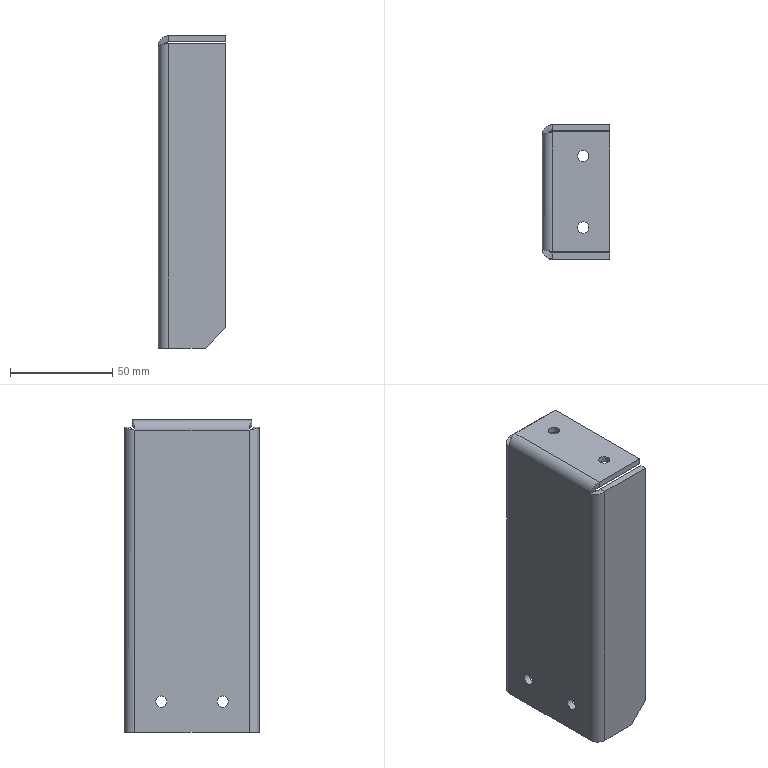Part | NX | 1 solid | 36 faces | box 33 x 66 x 153 mm | volume 60130 mm3 | plane 22 | cylinder 10 | spline 4 | commonest cylinder face diameters 5.5 x4 4 x3 10 x3
STEP:
#1=CARTESIAN_POINT('',(-3.,15.,-62.75));
#2=VERTEX_POINT('',#1);
#3=CARTESIAN_POINT('',(-3.,15.,-60.));
#4=DIRECTION('',(1.,0.,0.));
#5=DIRECTION('',(0.,0.,-1.));
#6=AXIS2_PLACEMENT_3D('',#3,#4,#5);
#7=CIRCLE('',#6,2.75);
#8=EDGE_CURVE('',#2,#2,#7,.T.);
#9=ORIENTED_EDGE('',*,*,#8,.T.);
#10=EDGE_LOOP('',(#9));
#11=FACE_BOUND('',#10,.T.);
#12=CARTESIAN_POINT('',(-3.,-15.,-62.75));
#13=VERTEX_POINT('',#12);
#14=CARTESIAN_POINT('',(-3.,-15.,-60.));
#15=DIRECTION('',(1.,0.,0.));
#16=DIRECTION('',(0.,0.,-1.));
#17=AXIS2_PLACEMENT_3D('',#14,#15,#16);
#18=CIRCLE('',#17,2.75);
#19=EDGE_CURVE('',#13,#13,#18,.T.);
#20=ORIENTED_EDGE('',*,*,#19,.T.);
#21=EDGE_LOOP('',(#20));
#22=FACE_BOUND('',#21,.T.);
#23=CARTESIAN_POINT('',(-3.,-28.,-75.));
#24=VERTEX_POINT('',#23);
#25=CARTESIAN_POINT('',(-3.,-28.,73.));
#26=VERTEX_POINT('',#25);
#27=CARTESIAN_POINT('',(-3.,-28.,-75.));
#28=DIRECTION('',(0.,0.,-1.));
#29=VECTOR('',#28,1000.);
#30=LINE('',#27,#29);
#31=EDGE_CURVE('',#24,#26,#30,.F.);
#32=ORIENTED_EDGE('',*,*,#31,.T.);
#33=CARTESIAN_POINT('',(-3.,28.,73.));
#34=VERTEX_POINT('',#33);
#35=CARTESIAN_POINT('',(-3.,-29.293,73.));
#36=DIRECTION('',(0.,-1.,0.));
#37=VECTOR('',#36,1000.);
#38=LINE('',#35,#37);
#39=EDGE_CURVE('',#26,#34,#38,.F.);
#40=ORIENTED_EDGE('',*,*,#39,.T.);
#41=CARTESIAN_POINT('',(-3.,28.,-75.));
#42=VERTEX_POINT('',#41);
#43=CARTESIAN_POINT('',(-3.,28.,74.293));
#44=DIRECTION('',(0.,0.,1.));
#45=VECTOR('',#44,1000.);
#46=LINE('',#43,#45);
#47=EDGE_CURVE('',#34,#42,#46,.F.);
#48=ORIENTED_EDGE('',*,*,#47,.T.);
#49=CARTESIAN_POINT('',(-3.,30.,-75.));
#50=DIRECTION('',(0.,1.,0.));
#51=VECTOR('',#50,1000.);
#52=LINE('',#49,#51);
#53=EDGE_CURVE('',#24,#42,#52,.T.);
#54=ORIENTED_EDGE('',*,*,#53,.F.);
#55=EDGE_LOOP('',(#32,#40,#48,#54));
#56=FACE_BOUND('',#55,.T.);
#57=CARTESIAN_POINT('',(-3.,0.,0.));
#58=DIRECTION('',(1.,0.,0.));
#59=DIRECTION('',(0.,0.,-1.));
#60=AXIS2_PLACEMENT_3D('',#57,#58,#59);
#61=PLANE('',#60);
#62=ADVANCED_FACE('',(#11,#22,#56),#61,.F.);
#63=CARTESIAN_POINT('',(0.,15.,-62.75));
#64=VERTEX_POINT('',#63);
#65=CARTESIAN_POINT('',(0.,15.,-60.));
#66=DIRECTION('',(1.,0.,0.));
#67=DIRECTION('',(0.,0.,-1.));
#68=AXIS2_PLACEMENT_3D('',#65,#66,#67);
#69=CIRCLE('',#68,2.75);
#70=EDGE_CURVE('',#64,#64,#69,.T.);
#71=ORIENTED_EDGE('',*,*,#70,.F.);
#72=EDGE_LOOP('',(#71));
#73=FACE_BOUND('',#72,.T.);
#74=CARTESIAN_POINT('',(0.,-15.,-62.75));
#75=VERTEX_POINT('',#74);
#76=CARTESIAN_POINT('',(0.,-15.,-60.));
#77=DIRECTION('',(1.,0.,0.));
#78=DIRECTION('',(0.,0.,-1.));
#79=AXIS2_PLACEMENT_3D('',#76,#77,#78);
#80=CIRCLE('',#79,2.75);
#81=EDGE_CURVE('',#75,#75,#80,.T.);
#82=ORIENTED_EDGE('',*,*,#81,.F.);
#83=EDGE_LOOP('',(#82));
#84=FACE_BOUND('',#83,.T.);
#85=CARTESIAN_POINT('',(0.,-28.,73.));
#86=VERTEX_POINT('',#85);
#87=CARTESIAN_POINT('',(0.,28.,73.));
#88=VERTEX_POINT('',#87);
#89=CARTESIAN_POINT('',(0.,-29.293,73.));
#90=DIRECTION('',(0.,-1.,0.));
#91=VECTOR('',#90,1000.);
#92=LINE('',#89,#91);
#93=EDGE_CURVE('',#86,#88,#92,.F.);
#94=ORIENTED_EDGE('',*,*,#93,.F.);
#95=CARTESIAN_POINT('',(0.,-28.,-75.));
#96=VERTEX_POINT('',#95);
#97=CARTESIAN_POINT('',(0.,-28.,-75.));
#98=DIRECTION('',(0.,0.,-1.));
#99=VECTOR('',#98,1000.);
#100=LINE('',#97,#99);
#101=EDGE_CURVE('',#96,#86,#100,.F.);
#102=ORIENTED_EDGE('',*,*,#101,.F.);
#103=CARTESIAN_POINT('',(0.,28.,-75.));
#104=VERTEX_POINT('',#103);
#105=CARTESIAN_POINT('',(0.,30.,-75.));
#106=DIRECTION('',(0.,1.,0.));
#107=VECTOR('',#106,1000.);
#108=LINE('',#105,#107);
#109=EDGE_CURVE('',#96,#104,#108,.T.);
#110=ORIENTED_EDGE('',*,*,#109,.T.);
#111=CARTESIAN_POINT('',(0.,28.,74.293));
#112=DIRECTION('',(0.,0.,1.));
#113=VECTOR('',#112,1000.);
#114=LINE('',#111,#113);
#115=EDGE_CURVE('',#88,#104,#114,.F.);
#116=ORIENTED_EDGE('',*,*,#115,.F.);
#117=EDGE_LOOP('',(#94,#102,#110,#116));
#118=FACE_BOUND('',#117,.T.);
#119=CARTESIAN_POINT('',(0.,0.,0.));
#120=DIRECTION('',(1.,0.,0.));
#121=DIRECTION('',(0.,0.,-1.));
#122=AXIS2_PLACEMENT_3D('',#119,#120,#121);
#123=PLANE('',#122);
#124=ADVANCED_FACE('',(#73,#84,#118),#123,.T.);
#125=ORIENTED_EDGE('',*,*,#109,.F.);
#126=CARTESIAN_POINT('',(0.,-28.,-75.));
#127=DIRECTION('',(-1.,0.,0.));
#128=VECTOR('',#127,1000.);
#129=LINE('',#126,#128);
#130=EDGE_CURVE('',#96,#24,#129,.T.);
#131=ORIENTED_EDGE('',*,*,#130,.T.);
#132=ORIENTED_EDGE('',*,*,#53,.T.);
#133=CARTESIAN_POINT('',(0.,28.,-75.));
#134=DIRECTION('',(-1.,0.,0.));
#135=VECTOR('',#134,1000.);
#136=LINE('',#133,#135);
#137=EDGE_CURVE('',#104,#42,#136,.T.);
#138=ORIENTED_EDGE('',*,*,#137,.F.);
#139=EDGE_LOOP('',(#125,#131,#132,#138));
#140=FACE_BOUND('',#139,.T.);
#141=CARTESIAN_POINT('',(-3.,30.,-75.));
#142=DIRECTION('',(0.,0.,-1.));
#143=DIRECTION('',(0.,1.,0.));
#144=AXIS2_PLACEMENT_3D('',#141,#142,#143);
#145=PLANE('',#144);
#146=ADVANCED_FACE('',(#140),#145,.T.);
#147=CARTESIAN_POINT('',(2.,29.293,78.));
#148=VERTEX_POINT('',#147);
#149=CARTESIAN_POINT('',(2.,29.293,75.));
#150=VERTEX_POINT('',#149);
#151=CARTESIAN_POINT('',(2.,29.293,75.));
#152=DIRECTION('',(0.,0.,-1.));
#153=VECTOR('',#152,1000.);
#154=LINE('',#151,#153);
#155=EDGE_CURVE('',#148,#150,#154,.T.);
#156=ORIENTED_EDGE('',*,*,#155,.T.);
#157=CARTESIAN_POINT('',(0.,28.,73.));
#158=CARTESIAN_POINT('',(0.,28.217,73.528));
#159=CARTESIAN_POINT('',(0.4352,28.646,74.564));
#160=CARTESIAN_POINT('',(1.472,29.075,75.));
#161=CARTESIAN_POINT('',(2.,29.293,75.));
#162=B_SPLINE_CURVE_WITH_KNOTS('',3,(#157,#158,#159,#160,#161),.UNSPECIFIED.,.F.,.F.,(4,1,4),(0.,0.00169,0.003379),.UNSPECIFIED.);
#163=EDGE_CURVE('',#88,#150,#162,.T.);
#164=ORIENTED_EDGE('',*,*,#163,.F.);
#165=CARTESIAN_POINT('',(0.,28.,73.));
#166=DIRECTION('',(-1.,0.,0.));
#167=VECTOR('',#166,1000.);
#168=LINE('',#165,#167);
#169=EDGE_CURVE('',#88,#34,#168,.T.);
#170=ORIENTED_EDGE('',*,*,#169,.T.);
#171=CARTESIAN_POINT('',(-3.,28.,73.));
#172=CARTESIAN_POINT('',(-3.,28.217,74.32));
#173=CARTESIAN_POINT('',(-1.912,28.646,76.91));
#174=CARTESIAN_POINT('',(0.6799,29.076,78.));
#175=CARTESIAN_POINT('',(2.,29.293,78.));
#176=B_SPLINE_CURVE_WITH_KNOTS('',3,(#171,#172,#173,#174,#175),.UNSPECIFIED.,.F.,.F.,(4,1,4),(0.,0.003969,0.007937),.UNSPECIFIED.);
#177=EDGE_CURVE('',#34,#148,#176,.T.);
#178=ORIENTED_EDGE('',*,*,#177,.T.);
#179=EDGE_LOOP('',(#156,#164,#170,#178));
#180=FACE_BOUND('',#179,.T.);
#181=CARTESIAN_POINT('',(-3.03,28.,73.));
#182=CARTESIAN_POINT('',(-3.03,28.108,73.659));
#183=CARTESIAN_POINT('',(-2.899,28.215,74.317));
#184=CARTESIAN_POINT('',(-2.395,28.431,75.533));
#185=CARTESIAN_POINT('',(-2.022,28.539,76.091));
#186=CARTESIAN_POINT('',(-1.091,28.754,77.022));
#187=CARTESIAN_POINT('',(-0.5332,28.862,77.395));
#188=CARTESIAN_POINT('',(0.6834,29.077,77.899));
#189=CARTESIAN_POINT('',(1.341,29.185,78.03));
#190=CARTESIAN_POINT('',(2.,29.293,78.03));
#191=CARTESIAN_POINT('',(-3.,28.,73.));
#192=CARTESIAN_POINT('',(-3.,28.108,73.655));
#193=CARTESIAN_POINT('',(-2.87,28.215,74.309));
#194=CARTESIAN_POINT('',(-2.369,28.431,75.518));
#195=CARTESIAN_POINT('',(-1.998,28.539,76.073));
#196=CARTESIAN_POINT('',(-1.073,28.754,76.998));
#197=CARTESIAN_POINT('',(-0.5181,28.862,77.369));
#198=CARTESIAN_POINT('',(0.6913,29.077,77.87));
#199=CARTESIAN_POINT('',(1.345,29.185,78.));
#200=CARTESIAN_POINT('',(2.,29.293,78.));
#201=CARTESIAN_POINT('',(0.,28.,73.));
#202=CARTESIAN_POINT('',(0.,28.108,73.262));
#203=CARTESIAN_POINT('',(0.05205,28.215,73.523));
#204=CARTESIAN_POINT('',(0.2524,28.431,74.007));
#205=CARTESIAN_POINT('',(0.4007,28.539,74.229));
#206=CARTESIAN_POINT('',(0.7709,28.754,74.599));
#207=CARTESIAN_POINT('',(0.9928,28.862,74.748));
#208=CARTESIAN_POINT('',(1.477,29.077,74.948));
#209=CARTESIAN_POINT('',(1.738,29.185,75.));
#210=CARTESIAN_POINT('',(2.,29.293,75.));
#211=CARTESIAN_POINT('',(0.0303,28.,73.));
#212=CARTESIAN_POINT('',(0.0303,28.108,73.258));
#213=CARTESIAN_POINT('',(0.08157,28.215,73.516));
#214=CARTESIAN_POINT('',(0.2789,28.431,73.992));
#215=CARTESIAN_POINT('',(0.4249,28.539,74.21));
#216=CARTESIAN_POINT('',(0.7895,28.754,74.575));
#217=CARTESIAN_POINT('',(1.008,28.862,74.721));
#218=CARTESIAN_POINT('',(1.484,29.077,74.918));
#219=CARTESIAN_POINT('',(1.742,29.185,74.97));
#220=CARTESIAN_POINT('',(2.,29.293,74.97));
#221=B_SPLINE_SURFACE_WITH_KNOTS('',1,3,((#181,#182,#183,#184,#185,#186,#187,#188,#189,#190),(#191,#192,#193,#194,#195,#196,#197,#198,#199,#200),(#201,#202,#203,#204,#205,#206,#207,#208,#209,#210),(#211,#212,#213,#214,#215,#216,#217,#218,#219,#220)),.RULED_SURF.,.F.,.F.,.F.,(2,1,1,2),(4,2,2,2,4),(-0.01,0.,1.,1.01),(0.,0.25,0.5,0.75,1.),.UNSPECIFIED.);
#222=ADVANCED_FACE('',(#180),#221,.F.);
#223=CARTESIAN_POINT('',(2.,-29.293,75.));
#224=VERTEX_POINT('',#223);
#225=CARTESIAN_POINT('',(2.,-29.293,75.));
#226=CARTESIAN_POINT('',(1.472,-29.075,75.));
#227=CARTESIAN_POINT('',(0.4362,-28.647,74.565));
#228=CARTESIAN_POINT('',(0.,-28.217,73.528));
#229=CARTESIAN_POINT('',(0.,-28.,73.));
#230=B_SPLINE_CURVE_WITH_KNOTS('',3,(#225,#226,#227,#228,#229),.UNSPECIFIED.,.F.,.F.,(4,1,4),(0.,0.00169,0.003379),.UNSPECIFIED.);
#231=EDGE_CURVE('',#224,#86,#230,.T.);
#232=ORIENTED_EDGE('',*,*,#231,.F.);
#233=CARTESIAN_POINT('',(2.,-29.293,78.));
#234=VERTEX_POINT('',#233);
#235=CARTESIAN_POINT('',(2.,-29.293,75.));
#236=DIRECTION('',(0.,0.,-1.));
#237=VECTOR('',#236,1000.);
#238=LINE('',#235,#237);
#239=EDGE_CURVE('',#234,#224,#238,.T.);
#240=ORIENTED_EDGE('',*,*,#239,.F.);
#241=CARTESIAN_POINT('',(2.,-29.293,78.));
#242=CARTESIAN_POINT('',(0.6799,-29.076,78.));
#243=CARTESIAN_POINT('',(-1.91,-28.647,76.912));
#244=CARTESIAN_POINT('',(-3.,-28.217,74.32));
#245=CARTESIAN_POINT('',(-3.,-28.,73.));
#246=B_SPLINE_CURVE_WITH_KNOTS('',3,(#241,#242,#243,#244,#245),.UNSPECIFIED.,.F.,.F.,(4,1,4),(0.,0.003969,0.007937),.UNSPECIFIED.);
#247=EDGE_CURVE('',#234,#26,#246,.T.);
#248=ORIENTED_EDGE('',*,*,#247,.T.);
#249=CARTESIAN_POINT('',(0.,-28.,73.));
#250=DIRECTION('',(-1.,0.,0.));
#251=VECTOR('',#250,1000.);
#252=LINE('',#249,#251);
#253=EDGE_CURVE('',#86,#26,#252,.T.);
#254=ORIENTED_EDGE('',*,*,#253,.F.);
#255=EDGE_LOOP('',(#232,#240,#248,#254));
#256=FACE_BOUND('',#255,.T.);
#257=CARTESIAN_POINT('',(2.,-29.293,78.03));
#258=CARTESIAN_POINT('',(1.341,-29.185,78.03));
#259=CARTESIAN_POINT('',(0.6834,-29.077,77.899));
#260=CARTESIAN_POINT('',(-0.5332,-28.862,77.395));
#261=CARTESIAN_POINT('',(-1.091,-28.754,77.022));
#262=CARTESIAN_POINT('',(-2.022,-28.539,76.091));
#263=CARTESIAN_POINT('',(-2.395,-28.431,75.533));
#264=CARTESIAN_POINT('',(-2.899,-28.215,74.317));
#265=CARTESIAN_POINT('',(-3.03,-28.108,73.659));
#266=CARTESIAN_POINT('',(-3.03,-28.,73.));
#267=CARTESIAN_POINT('',(2.,-29.293,78.));
#268=CARTESIAN_POINT('',(1.345,-29.185,78.));
#269=CARTESIAN_POINT('',(0.6913,-29.077,77.87));
#270=CARTESIAN_POINT('',(-0.5181,-28.862,77.369));
#271=CARTESIAN_POINT('',(-1.073,-28.754,76.998));
#272=CARTESIAN_POINT('',(-1.998,-28.539,76.073));
#273=CARTESIAN_POINT('',(-2.369,-28.431,75.518));
#274=CARTESIAN_POINT('',(-2.87,-28.215,74.309));
#275=CARTESIAN_POINT('',(-3.,-28.108,73.655));
#276=CARTESIAN_POINT('',(-3.,-28.,73.));
#277=CARTESIAN_POINT('',(2.,-29.293,75.));
#278=CARTESIAN_POINT('',(1.738,-29.185,75.));
#279=CARTESIAN_POINT('',(1.477,-29.077,74.948));
#280=CARTESIAN_POINT('',(0.9928,-28.862,74.748));
#281=CARTESIAN_POINT('',(0.7709,-28.754,74.599));
#282=CARTESIAN_POINT('',(0.4007,-28.539,74.229));
#283=CARTESIAN_POINT('',(0.2524,-28.431,74.007));
#284=CARTESIAN_POINT('',(0.05205,-28.215,73.523));
#285=CARTESIAN_POINT('',(0.,-28.108,73.262));
#286=CARTESIAN_POINT('',(0.,-28.,73.));
#287=CARTESIAN_POINT('',(2.,-29.293,74.97));
#288=CARTESIAN_POINT('',(1.742,-29.185,74.97));
#289=CARTESIAN_POINT('',(1.484,-29.077,74.918));
#290=CARTESIAN_POINT('',(1.008,-28.862,74.721));
#291=CARTESIAN_POINT('',(0.7895,-28.754,74.575));
#292=CARTESIAN_POINT('',(0.4249,-28.539,74.21));
#293=CARTESIAN_POINT('',(0.2789,-28.431,73.992));
#294=CARTESIAN_POINT('',(0.08157,-28.215,73.516));
#295=CARTESIAN_POINT('',(0.0303,-28.108,73.258));
#296=CARTESIAN_POINT('',(0.0303,-28.,73.));
#297=B_SPLINE_SURFACE_WITH_KNOTS('',1,3,((#257,#258,#259,#260,#261,#262,#263,#264,#265,#266),(#267,#268,#269,#270,#271,#272,#273,#274,#275,#276),(#277,#278,#279,#280,#281,#282,#283,#284,#285,#286),(#287,#288,#289,#290,#291,#292,#293,#294,#295,#296)),.RULED_SURF.,.F.,.F.,.F.,(2,1,1,2),(4,2,2,2,4),(-0.01,0.,1.,1.01),(0.,0.25,0.5,0.75,1.),.UNSPECIFIED.);
#298=ADVANCED_FACE('',(#256),#297,.F.);
#299=ORIENTED_EDGE('',*,*,#39,.F.);
#300=ORIENTED_EDGE('',*,*,#247,.F.);
#301=CARTESIAN_POINT('',(2.,0.,78.));
#302=DIRECTION('',(0.,1.,0.));
#303=VECTOR('',#302,1000.);
#304=LINE('',#301,#303);
#305=EDGE_CURVE('',#234,#148,#304,.T.);
#306=ORIENTED_EDGE('',*,*,#305,.T.);
#307=ORIENTED_EDGE('',*,*,#177,.F.);
#308=EDGE_LOOP('',(#299,#300,#306,#307));
#309=FACE_BOUND('',#308,.T.);
#310=CARTESIAN_POINT('',(2.,-29.293,73.));
#311=DIRECTION('',(0.,-1.,0.));
#312=DIRECTION('',(0.,0.,1.));
#313=AXIS2_PLACEMENT_3D('',#310,#311,#312);
#314=CYLINDRICAL_SURFACE('',#313,5.);
#315=ADVANCED_FACE('',(#309),#314,.T.);
#316=ORIENTED_EDGE('',*,*,#93,.T.);
#317=ORIENTED_EDGE('',*,*,#163,.T.);
#318=CARTESIAN_POINT('',(2.,30.,75.));
#319=DIRECTION('',(0.,-1.,0.));
#320=VECTOR('',#319,1000.);
#321=LINE('',#318,#320);
#322=EDGE_CURVE('',#150,#224,#321,.T.);
#323=ORIENTED_EDGE('',*,*,#322,.T.);
#324=ORIENTED_EDGE('',*,*,#231,.T.);
#325=EDGE_LOOP('',(#316,#317,#323,#324));
#326=FACE_BOUND('',#325,.T.);
#327=CARTESIAN_POINT('',(2.,-29.293,73.));
#328=DIRECTION('',(0.,-1.,0.));
#329=DIRECTION('',(0.,0.,1.));
#330=AXIS2_PLACEMENT_3D('',#327,#328,#329);
#331=CYLINDRICAL_SURFACE('',#330,2.);
#332=ADVANCED_FACE('',(#326),#331,.F.);
#333=CARTESIAN_POINT('',(30.,29.293,78.));
#334=VERTEX_POINT('',#333);
#335=CARTESIAN_POINT('',(0.,29.293,78.));
#336=DIRECTION('',(1.,0.,0.));
#337=VECTOR('',#336,1000.);
#338=LINE('',#335,#337);
#339=EDGE_CURVE('',#148,#334,#338,.T.);
#340=ORIENTED_EDGE('',*,*,#339,.T.);
#341=CARTESIAN_POINT('',(30.,29.293,75.));
#342=VERTEX_POINT('',#341);
#343=CARTESIAN_POINT('',(30.,29.293,78.));
#344=DIRECTION('',(0.,0.,-1.));
#345=VECTOR('',#344,1000.);
#346=LINE('',#343,#345);
#347=EDGE_CURVE('',#334,#342,#346,.T.);
#348=ORIENTED_EDGE('',*,*,#347,.T.);
#349=CARTESIAN_POINT('',(0.,29.293,75.));
#350=DIRECTION('',(1.,0.,0.));
#351=VECTOR('',#350,1000.);
#352=LINE('',#349,#351);
#353=EDGE_CURVE('',#150,#342,#352,.T.);
#354=ORIENTED_EDGE('',*,*,#353,.F.);
#355=ORIENTED_EDGE('',*,*,#155,.F.);
#356=EDGE_LOOP('',(#340,#348,#354,#355));
#357=FACE_BOUND('',#356,.T.);
#358=CARTESIAN_POINT('',(0.,29.293,75.));
#359=DIRECTION('',(0.,1.,0.));
#360=DIRECTION('',(-1.,0.,0.));
#361=AXIS2_PLACEMENT_3D('',#358,#359,#360);
#362=PLANE('',#361);
#363=ADVANCED_FACE('',(#357),#362,.T.);
#364=CARTESIAN_POINT('',(19.75,17.5,78.));
#365=VERTEX_POINT('',#364);
#366=CARTESIAN_POINT('',(17.,17.5,78.));
#367=DIRECTION('',(0.,0.,1.));
#368=DIRECTION('',(1.,0.,0.));
#369=AXIS2_PLACEMENT_3D('',#366,#367,#368);
#370=CIRCLE('',#369,2.75);
#371=EDGE_CURVE('',#365,#365,#370,.T.);
#372=ORIENTED_EDGE('',*,*,#371,.F.);
#373=EDGE_LOOP('',(#372));
#374=FACE_BOUND('',#373,.T.);
#375=CARTESIAN_POINT('',(19.75,-17.5,78.));
#376=VERTEX_POINT('',#375);
#377=CARTESIAN_POINT('',(17.,-17.5,78.));
#378=DIRECTION('',(0.,0.,1.));
#379=DIRECTION('',(1.,0.,0.));
#380=AXIS2_PLACEMENT_3D('',#377,#378,#379);
#381=CIRCLE('',#380,2.75);
#382=EDGE_CURVE('',#376,#376,#381,.T.);
#383=ORIENTED_EDGE('',*,*,#382,.F.);
#384=EDGE_LOOP('',(#383));
#385=FACE_BOUND('',#384,.T.);
#386=ORIENTED_EDGE('',*,*,#305,.F.);
#387=CARTESIAN_POINT('',(30.,-29.293,78.));
#388=VERTEX_POINT('',#387);
#389=CARTESIAN_POINT('',(0.,-29.293,78.));
#390=DIRECTION('',(1.,0.,0.));
#391=VECTOR('',#390,1000.);
#392=LINE('',#389,#391);
#393=EDGE_CURVE('',#234,#388,#392,.T.);
#394=ORIENTED_EDGE('',*,*,#393,.T.);
#395=CARTESIAN_POINT('',(30.,30.,78.));
#396=DIRECTION('',(0.,1.,0.));
#397=VECTOR('',#396,1000.);
#398=LINE('',#395,#397);
#399=EDGE_CURVE('',#388,#334,#398,.T.);
#400=ORIENTED_EDGE('',*,*,#399,.T.);
#401=ORIENTED_EDGE('',*,*,#339,.F.);
#402=EDGE_LOOP('',(#386,#394,#400,#401));
#403=FACE_BOUND('',#402,.T.);
#404=CARTESIAN_POINT('',(0.,0.,78.));
#405=DIRECTION('',(0.,0.,-1.));
#406=DIRECTION('',(-1.,0.,0.));
#407=AXIS2_PLACEMENT_3D('',#404,#405,#406);
#408=PLANE('',#407);
#409=ADVANCED_FACE('',(#374,#385,#403),#408,.F.);
#410=CARTESIAN_POINT('',(14.25,17.5,75.));
#411=VERTEX_POINT('',#410);
#412=CARTESIAN_POINT('',(17.,17.5,75.));
#413=DIRECTION('',(0.,0.,-1.));
#414=DIRECTION('',(-1.,0.,0.));
#415=AXIS2_PLACEMENT_3D('',#412,#413,#414);
#416=CIRCLE('',#415,2.75);
#417=EDGE_CURVE('',#411,#411,#416,.T.);
#418=ORIENTED_EDGE('',*,*,#417,.F.);
#419=EDGE_LOOP('',(#418));
#420=FACE_BOUND('',#419,.T.);
#421=CARTESIAN_POINT('',(14.25,-17.5,75.));
#422=VERTEX_POINT('',#421);
#423=CARTESIAN_POINT('',(17.,-17.5,75.));
#424=DIRECTION('',(0.,0.,-1.));
#425=DIRECTION('',(-1.,0.,0.));
#426=AXIS2_PLACEMENT_3D('',#423,#424,#425);
#427=CIRCLE('',#426,2.75);
#428=EDGE_CURVE('',#422,#422,#427,.T.);
#429=ORIENTED_EDGE('',*,*,#428,.F.);
#430=EDGE_LOOP('',(#429));
#431=FACE_BOUND('',#430,.T.);
#432=CARTESIAN_POINT('',(30.,-29.293,75.));
#433=VERTEX_POINT('',#432);
#434=CARTESIAN_POINT('',(0.,-29.293,75.));
#435=DIRECTION('',(1.,0.,0.));
#436=VECTOR('',#435,1000.);
#437=LINE('',#434,#436);
#438=EDGE_CURVE('',#224,#433,#437,.T.);
#439=ORIENTED_EDGE('',*,*,#438,.F.);
#440=ORIENTED_EDGE('',*,*,#322,.F.);
#441=ORIENTED_EDGE('',*,*,#353,.T.);
#442=CARTESIAN_POINT('',(30.,30.,75.));
#443=DIRECTION('',(0.,1.,0.));
#444=VECTOR('',#443,1000.);
#445=LINE('',#442,#444);
#446=EDGE_CURVE('',#433,#342,#445,.T.);
#447=ORIENTED_EDGE('',*,*,#446,.F.);
#448=EDGE_LOOP('',(#439,#440,#441,#447));
#449=FACE_BOUND('',#448,.T.);
#450=CARTESIAN_POINT('',(0.,0.,75.));
#451=DIRECTION('',(0.,0.,-1.));
#452=DIRECTION('',(-1.,0.,0.));
#453=AXIS2_PLACEMENT_3D('',#450,#451,#452);
#454=PLANE('',#453);
#455=ADVANCED_FACE('',(#420,#431,#449),#454,.T.);
#456=ORIENTED_EDGE('',*,*,#399,.F.);
#457=CARTESIAN_POINT('',(30.,-29.293,78.));
#458=DIRECTION('',(0.,0.,-1.));
#459=VECTOR('',#458,1000.);
#460=LINE('',#457,#459);
#461=EDGE_CURVE('',#388,#433,#460,.T.);
#462=ORIENTED_EDGE('',*,*,#461,.T.);
#463=ORIENTED_EDGE('',*,*,#446,.T.);
#464=ORIENTED_EDGE('',*,*,#347,.F.);
#465=EDGE_LOOP('',(#456,#462,#463,#464));
#466=FACE_BOUND('',#465,.T.);
#467=CARTESIAN_POINT('',(30.,30.,78.));
#468=DIRECTION('',(-1.,0.,0.));
#469=DIRECTION('',(0.,0.,1.));
#470=AXIS2_PLACEMENT_3D('',#467,#468,#469);
#471=PLANE('',#470);
#472=ADVANCED_FACE('',(#466),#471,.F.);
#473=ORIENTED_EDGE('',*,*,#461,.F.);
#474=ORIENTED_EDGE('',*,*,#393,.F.);
#475=ORIENTED_EDGE('',*,*,#239,.T.);
#476=ORIENTED_EDGE('',*,*,#438,.T.);
#477=EDGE_LOOP('',(#473,#474,#475,#476));
#478=FACE_BOUND('',#477,.T.);
#479=CARTESIAN_POINT('',(0.,-29.293,75.));
#480=DIRECTION('',(0.,1.,0.));
#481=DIRECTION('',(-1.,0.,0.));
#482=AXIS2_PLACEMENT_3D('',#479,#480,#481);
#483=PLANE('',#482);
#484=ADVANCED_FACE('',(#478),#483,.F.);
#485=CARTESIAN_POINT('',(2.,30.,-75.));
#486=VERTEX_POINT('',#485);
#487=CARTESIAN_POINT('',(2.,33.,-75.));
#488=VERTEX_POINT('',#487);
#489=CARTESIAN_POINT('',(2.,30.,-75.));
#490=DIRECTION('',(0.,1.,0.));
#491=VECTOR('',#490,1000.);
#492=LINE('',#489,#491);
#493=EDGE_CURVE('',#486,#488,#492,.T.);
#494=ORIENTED_EDGE('',*,*,#493,.F.);
#495=CARTESIAN_POINT('',(2.,28.,-75.));
#496=DIRECTION('',(0.,0.,1.));
#497=DIRECTION('',(1.,0.,0.));
#498=AXIS2_PLACEMENT_3D('',#495,#496,#497);
#499=CIRCLE('',#498,2.);
#500=EDGE_CURVE('',#104,#486,#499,.F.);
#501=ORIENTED_EDGE('',*,*,#500,.F.);
#502=ORIENTED_EDGE('',*,*,#137,.T.);
#503=CARTESIAN_POINT('',(2.,28.,-75.));
#504=DIRECTION('',(0.,0.,1.));
#505=DIRECTION('',(1.,0.,0.));
#506=AXIS2_PLACEMENT_3D('',#503,#504,#505);
#507=CIRCLE('',#506,5.);
#508=EDGE_CURVE('',#42,#488,#507,.F.);
#509=ORIENTED_EDGE('',*,*,#508,.T.);
#510=EDGE_LOOP('',(#494,#501,#502,#509));
#511=FACE_BOUND('',#510,.T.);
#512=CARTESIAN_POINT('',(2.,28.,-75.));
#513=DIRECTION('',(0.,0.,-1.));
#514=DIRECTION('',(-1.,0.,0.));
#515=AXIS2_PLACEMENT_3D('',#512,#513,#514);
#516=PLANE('',#515);
#517=ADVANCED_FACE('',(#511),#516,.T.);
#518=CARTESIAN_POINT('',(2.,30.,74.293));
#519=VERTEX_POINT('',#518);
#520=CARTESIAN_POINT('',(2.,30.,74.293));
#521=CARTESIAN_POINT('',(1.472,30.,74.075));
#522=CARTESIAN_POINT('',(0.4362,29.565,73.647));
#523=CARTESIAN_POINT('',(0.,28.528,73.217));
#524=CARTESIAN_POINT('',(0.,28.,73.));
#525=B_SPLINE_CURVE_WITH_KNOTS('',3,(#520,#521,#522,#523,#524),.UNSPECIFIED.,.F.,.F.,(4,1,4),(0.,0.00169,0.003379),.UNSPECIFIED.);
#526=EDGE_CURVE('',#519,#88,#525,.T.);
#527=ORIENTED_EDGE('',*,*,#526,.F.);
#528=CARTESIAN_POINT('',(2.,33.,74.293));
#529=VERTEX_POINT('',#528);
#530=CARTESIAN_POINT('',(2.,30.,74.293));
#531=DIRECTION('',(0.,-1.,0.));
#532=VECTOR('',#531,1000.);
#533=LINE('',#530,#532);
#534=EDGE_CURVE('',#529,#519,#533,.T.);
#535=ORIENTED_EDGE('',*,*,#534,.F.);
#536=CARTESIAN_POINT('',(2.,33.,74.293));
#537=CARTESIAN_POINT('',(0.6799,33.,74.076));
#538=CARTESIAN_POINT('',(-1.91,31.912,73.647));
#539=CARTESIAN_POINT('',(-3.,29.32,73.217));
#540=CARTESIAN_POINT('',(-3.,28.,73.));
#541=B_SPLINE_CURVE_WITH_KNOTS('',3,(#536,#537,#538,#539,#540),.UNSPECIFIED.,.F.,.F.,(4,1,4),(0.,0.003969,0.007937),.UNSPECIFIED.);
#542=EDGE_CURVE('',#529,#34,#541,.T.);
#543=ORIENTED_EDGE('',*,*,#542,.T.);
#544=ORIENTED_EDGE('',*,*,#169,.F.);
#545=EDGE_LOOP('',(#527,#535,#543,#544));
#546=FACE_BOUND('',#545,.T.);
#547=CARTESIAN_POINT('',(2.,33.03,74.293));
#548=CARTESIAN_POINT('',(1.341,33.03,74.185));
#549=CARTESIAN_POINT('',(0.6834,32.899,74.077));
#550=CARTESIAN_POINT('',(-0.5332,32.395,73.862));
#551=CARTESIAN_POINT('',(-1.091,32.022,73.754));
#552=CARTESIAN_POINT('',(-2.022,31.091,73.539));
#553=CARTESIAN_POINT('',(-2.395,30.533,73.431));
#554=CARTESIAN_POINT('',(-2.899,29.317,73.215));
#555=CARTESIAN_POINT('',(-3.03,28.659,73.108));
#556=CARTESIAN_POINT('',(-3.03,28.,73.));
#557=CARTESIAN_POINT('',(2.,33.,74.293));
#558=CARTESIAN_POINT('',(1.345,33.,74.185));
#559=CARTESIAN_POINT('',(0.6913,32.87,74.077));
#560=CARTESIAN_POINT('',(-0.5181,32.369,73.862));
#561=CARTESIAN_POINT('',(-1.073,31.998,73.754));
#562=CARTESIAN_POINT('',(-1.998,31.073,73.539));
#563=CARTESIAN_POINT('',(-2.369,30.518,73.431));
#564=CARTESIAN_POINT('',(-2.87,29.309,73.215));
#565=CARTESIAN_POINT('',(-3.,28.655,73.108));
#566=CARTESIAN_POINT('',(-3.,28.,73.));
#567=CARTESIAN_POINT('',(2.,30.,74.293));
#568=CARTESIAN_POINT('',(1.738,30.,74.185));
#569=CARTESIAN_POINT('',(1.477,29.948,74.077));
#570=CARTESIAN_POINT('',(0.9928,29.748,73.862));
#571=CARTESIAN_POINT('',(0.7709,29.599,73.754));
#572=CARTESIAN_POINT('',(0.4007,29.229,73.539));
#573=CARTESIAN_POINT('',(0.2524,29.007,73.431));
#574=CARTESIAN_POINT('',(0.05205,28.523,73.215));
#575=CARTESIAN_POINT('',(0.,28.262,73.108));
#576=CARTESIAN_POINT('',(0.,28.,73.));
#577=CARTESIAN_POINT('',(2.,29.97,74.293));
#578=CARTESIAN_POINT('',(1.742,29.97,74.185));
#579=CARTESIAN_POINT('',(1.484,29.918,74.077));
#580=CARTESIAN_POINT('',(1.008,29.721,73.862));
#581=CARTESIAN_POINT('',(0.7895,29.575,73.754));
#582=CARTESIAN_POINT('',(0.4249,29.21,73.539));
#583=CARTESIAN_POINT('',(0.2789,28.992,73.431));
#584=CARTESIAN_POINT('',(0.08157,28.516,73.215));
#585=CARTESIAN_POINT('',(0.0303,28.258,73.108));
#586=CARTESIAN_POINT('',(0.0303,28.,73.));
#587=B_SPLINE_SURFACE_WITH_KNOTS('',1,3,((#547,#548,#549,#550,#551,#552,#553,#554,#555,#556),(#557,#558,#559,#560,#561,#562,#563,#564,#565,#566),(#567,#568,#569,#570,#571,#572,#573,#574,#575,#576),(#577,#578,#579,#580,#581,#582,#583,#584,#585,#586)),.RULED_SURF.,.F.,.F.,.F.,(2,1,1,2),(4,2,2,2,4),(-0.01,0.,1.,1.01),(0.,0.25,0.5,0.75,1.),.UNSPECIFIED.);
#588=ADVANCED_FACE('',(#546),#587,.F.);
#589=ORIENTED_EDGE('',*,*,#47,.F.);
#590=ORIENTED_EDGE('',*,*,#542,.F.);
#591=CARTESIAN_POINT('',(2.,33.,0.));
#592=DIRECTION('',(0.,0.,-1.));
#593=VECTOR('',#592,1000.);
#594=LINE('',#591,#593);
#595=EDGE_CURVE('',#529,#488,#594,.T.);
#596=ORIENTED_EDGE('',*,*,#595,.T.);
#597=ORIENTED_EDGE('',*,*,#508,.F.);
#598=EDGE_LOOP('',(#589,#590,#596,#597));
#599=FACE_BOUND('',#598,.T.);
#600=CARTESIAN_POINT('',(2.,28.,74.293));
#601=DIRECTION('',(0.,0.,1.));
#602=DIRECTION('',(0.,1.,0.));
#603=AXIS2_PLACEMENT_3D('',#600,#601,#602);
#604=CYLINDRICAL_SURFACE('',#603,5.);
#605=ADVANCED_FACE('',(#599),#604,.T.);
#606=ORIENTED_EDGE('',*,*,#115,.T.);
#607=ORIENTED_EDGE('',*,*,#500,.T.);
#608=CARTESIAN_POINT('',(2.,30.,-75.));
#609=DIRECTION('',(0.,0.,1.));
#610=VECTOR('',#609,1000.);
#611=LINE('',#608,#610);
#612=EDGE_CURVE('',#486,#519,#611,.T.);
#613=ORIENTED_EDGE('',*,*,#612,.T.);
#614=ORIENTED_EDGE('',*,*,#526,.T.);
#615=EDGE_LOOP('',(#606,#607,#613,#614));
#616=FACE_BOUND('',#615,.T.);
#617=CARTESIAN_POINT('',(2.,28.,74.293));
#618=DIRECTION('',(0.,0.,1.));
#619=DIRECTION('',(0.,1.,0.));
#620=AXIS2_PLACEMENT_3D('',#617,#618,#619);
#621=CYLINDRICAL_SURFACE('',#620,2.);
#622=ADVANCED_FACE('',(#616),#621,.F.);
#623=CARTESIAN_POINT('',(20.,33.,-75.));
#624=VERTEX_POINT('',#623);
#625=CARTESIAN_POINT('',(0.,33.,-75.));
#626=DIRECTION('',(-1.,0.,0.));
#627=VECTOR('',#626,1000.);
#628=LINE('',#625,#627);
#629=EDGE_CURVE('',#624,#488,#628,.T.);
#630=ORIENTED_EDGE('',*,*,#629,.F.);
#631=CARTESIAN_POINT('',(20.,30.,-75.));
#632=VERTEX_POINT('',#631);
#633=CARTESIAN_POINT('',(20.,33.,-75.));
#634=DIRECTION('',(0.,-1.,0.));
#635=VECTOR('',#634,1000.);
#636=LINE('',#633,#635);
#637=EDGE_CURVE('',#624,#632,#636,.T.);
#638=ORIENTED_EDGE('',*,*,#637,.T.);
#639=CARTESIAN_POINT('',(0.,30.,-75.));
#640=DIRECTION('',(-1.,0.,0.));
#641=VECTOR('',#640,1000.);
#642=LINE('',#639,#641);
#643=EDGE_CURVE('',#632,#486,#642,.T.);
#644=ORIENTED_EDGE('',*,*,#643,.T.);
#645=ORIENTED_EDGE('',*,*,#493,.T.);
#646=EDGE_LOOP('',(#630,#638,#644,#645));
#647=FACE_BOUND('',#646,.T.);
#648=CARTESIAN_POINT('',(0.,33.,-75.));
#649=DIRECTION('',(0.,0.,1.));
#650=DIRECTION('',(1.,0.,0.));
#651=AXIS2_PLACEMENT_3D('',#648,#649,#650);
#652=PLANE('',#651);
#653=ADVANCED_FACE('',(#647),#652,.F.);
#654=CARTESIAN_POINT('',(30.,33.,74.293));
#655=VERTEX_POINT('',#654);
#656=CARTESIAN_POINT('',(30.,33.,-65.));
#657=VERTEX_POINT('',#656);
#658=CARTESIAN_POINT('',(30.,33.,-75.));
#659=DIRECTION('',(0.,0.,-1.));
#660=VECTOR('',#659,1000.);
#661=LINE('',#658,#660);
#662=EDGE_CURVE('',#655,#657,#661,.T.);
#663=ORIENTED_EDGE('',*,*,#662,.T.);
#664=CARTESIAN_POINT('',(20.,33.,-75.));
#665=DIRECTION('',(0.7071,0.,0.7071));
#666=VECTOR('',#665,1000.);
#667=LINE('',#664,#666);
#668=EDGE_CURVE('',#657,#624,#667,.F.);
#669=ORIENTED_EDGE('',*,*,#668,.T.);
#670=ORIENTED_EDGE('',*,*,#629,.T.);
#671=ORIENTED_EDGE('',*,*,#595,.F.);
#672=CARTESIAN_POINT('',(0.,33.,74.293));
#673=DIRECTION('',(1.,0.,0.));
#674=VECTOR('',#673,1000.);
#675=LINE('',#672,#674);
#676=EDGE_CURVE('',#529,#655,#675,.T.);
#677=ORIENTED_EDGE('',*,*,#676,.T.);
#678=EDGE_LOOP('',(#663,#669,#670,#671,#677));
#679=FACE_BOUND('',#678,.T.);
#680=CARTESIAN_POINT('',(0.,33.,0.));
#681=DIRECTION('',(0.,-1.,0.));
#682=DIRECTION('',(1.,0.,0.));
#683=AXIS2_PLACEMENT_3D('',#680,#681,#682);
#684=PLANE('',#683);
#685=ADVANCED_FACE('',(#679),#684,.F.);
#686=ORIENTED_EDGE('',*,*,#643,.F.);
#687=CARTESIAN_POINT('',(30.,30.,-65.));
#688=VERTEX_POINT('',#687);
#689=CARTESIAN_POINT('',(47.5,30.,-47.5));
#690=DIRECTION('',(-0.7071,0.,-0.7071));
#691=VECTOR('',#690,1000.);
#692=LINE('',#689,#691);
#693=EDGE_CURVE('',#632,#688,#692,.F.);
#694=ORIENTED_EDGE('',*,*,#693,.T.);
#695=CARTESIAN_POINT('',(30.,30.,74.293));
#696=VERTEX_POINT('',#695);
#697=CARTESIAN_POINT('',(30.,30.,-75.));
#698=DIRECTION('',(0.,0.,-1.));
#699=VECTOR('',#698,1000.);
#700=LINE('',#697,#699);
#701=EDGE_CURVE('',#696,#688,#700,.T.);
#702=ORIENTED_EDGE('',*,*,#701,.F.);
#703=CARTESIAN_POINT('',(0.,30.,74.293));
#704=DIRECTION('',(1.,0.,0.));
#705=VECTOR('',#704,1000.);
#706=LINE('',#703,#705);
#707=EDGE_CURVE('',#519,#696,#706,.T.);
#708=ORIENTED_EDGE('',*,*,#707,.F.);
#709=ORIENTED_EDGE('',*,*,#612,.F.);
#710=EDGE_LOOP('',(#686,#694,#702,#708,#709));
#711=FACE_BOUND('',#710,.T.);
#712=CARTESIAN_POINT('',(0.,30.,0.));
#713=DIRECTION('',(0.,-1.,0.));
#714=DIRECTION('',(1.,0.,0.));
#715=AXIS2_PLACEMENT_3D('',#712,#713,#714);
#716=PLANE('',#715);
#717=ADVANCED_FACE('',(#711),#716,.T.);
#718=ORIENTED_EDGE('',*,*,#701,.T.);
#719=CARTESIAN_POINT('',(30.,33.,-65.));
#720=DIRECTION('',(0.,1.,0.));
#721=VECTOR('',#720,1000.);
#722=LINE('',#719,#721);
#723=EDGE_CURVE('',#688,#657,#722,.T.);
#724=ORIENTED_EDGE('',*,*,#723,.T.);
#725=ORIENTED_EDGE('',*,*,#662,.F.);
#726=CARTESIAN_POINT('',(30.,33.,74.293));
#727=DIRECTION('',(0.,-1.,0.));
#728=VECTOR('',#727,1000.);
#729=LINE('',#726,#728);
#730=EDGE_CURVE('',#655,#696,#729,.T.);
#731=ORIENTED_EDGE('',*,*,#730,.T.);
#732=EDGE_LOOP('',(#718,#724,#725,#731));
#733=FACE_BOUND('',#732,.T.);
#734=CARTESIAN_POINT('',(30.,33.,-75.));
#735=DIRECTION('',(-1.,0.,0.));
#736=DIRECTION('',(0.,-1.,0.));
#737=AXIS2_PLACEMENT_3D('',#734,#735,#736);
#738=PLANE('',#737);
#739=ADVANCED_FACE('',(#733),#738,.F.);
#740=ORIENTED_EDGE('',*,*,#730,.F.);
#741=ORIENTED_EDGE('',*,*,#676,.F.);
#742=ORIENTED_EDGE('',*,*,#534,.T.);
#743=ORIENTED_EDGE('',*,*,#707,.T.);
#744=EDGE_LOOP('',(#740,#741,#742,#743));
#745=FACE_BOUND('',#744,.T.);
#746=CARTESIAN_POINT('',(0.,30.,74.293));
#747=DIRECTION('',(0.,0.,-1.));
#748=DIRECTION('',(-1.,0.,0.));
#749=AXIS2_PLACEMENT_3D('',#746,#747,#748);
#750=PLANE('',#749);
#751=ADVANCED_FACE('',(#745),#750,.F.);
#752=CARTESIAN_POINT('',(2.,-33.,74.293));
#753=VERTEX_POINT('',#752);
#754=CARTESIAN_POINT('',(2.,-30.,74.293));
#755=VERTEX_POINT('',#754);
#756=CARTESIAN_POINT('',(2.,-30.,74.293));
#757=DIRECTION('',(0.,1.,0.));
#758=VECTOR('',#757,1000.);
#759=LINE('',#756,#758);
#760=EDGE_CURVE('',#753,#755,#759,.T.);
#761=ORIENTED_EDGE('',*,*,#760,.T.);
#762=CARTESIAN_POINT('',(0.,-28.,73.));
#763=CARTESIAN_POINT('',(0.,-28.528,73.217));
#764=CARTESIAN_POINT('',(0.4352,-29.564,73.646));
#765=CARTESIAN_POINT('',(1.472,-30.,74.075));
#766=CARTESIAN_POINT('',(2.,-30.,74.293));
#767=B_SPLINE_CURVE_WITH_KNOTS('',3,(#762,#763,#764,#765,#766),.UNSPECIFIED.,.F.,.F.,(4,1,4),(0.,0.00169,0.003379),.UNSPECIFIED.);
#768=EDGE_CURVE('',#86,#755,#767,.T.);
#769=ORIENTED_EDGE('',*,*,#768,.F.);
#770=ORIENTED_EDGE('',*,*,#253,.T.);
#771=CARTESIAN_POINT('',(-3.,-28.,73.));
#772=CARTESIAN_POINT('',(-3.,-29.32,73.217));
#773=CARTESIAN_POINT('',(-1.912,-31.91,73.646));
#774=CARTESIAN_POINT('',(0.6799,-33.,74.076));
#775=CARTESIAN_POINT('',(2.,-33.,74.293));
#776=B_SPLINE_CURVE_WITH_KNOTS('',3,(#771,#772,#773,#774,#775),.UNSPECIFIED.,.F.,.F.,(4,1,4),(0.,0.003969,0.007937),.UNSPECIFIED.);
#777=EDGE_CURVE('',#26,#753,#776,.T.);
#778=ORIENTED_EDGE('',*,*,#777,.T.);
#779=EDGE_LOOP('',(#761,#769,#770,#778));
#780=FACE_BOUND('',#779,.T.);
#781=CARTESIAN_POINT('',(-3.03,-28.,73.));
#782=CARTESIAN_POINT('',(-3.03,-28.659,73.108));
#783=CARTESIAN_POINT('',(-2.899,-29.317,73.215));
#784=CARTESIAN_POINT('',(-2.395,-30.533,73.431));
#785=CARTESIAN_POINT('',(-2.022,-31.091,73.539));
#786=CARTESIAN_POINT('',(-1.091,-32.022,73.754));
#787=CARTESIAN_POINT('',(-0.5332,-32.395,73.862));
#788=CARTESIAN_POINT('',(0.6834,-32.899,74.077));
#789=CARTESIAN_POINT('',(1.341,-33.03,74.185));
#790=CARTESIAN_POINT('',(2.,-33.03,74.293));
#791=CARTESIAN_POINT('',(-3.,-28.,73.));
#792=CARTESIAN_POINT('',(-3.,-28.655,73.108));
#793=CARTESIAN_POINT('',(-2.87,-29.309,73.215));
#794=CARTESIAN_POINT('',(-2.369,-30.518,73.431));
#795=CARTESIAN_POINT('',(-1.998,-31.073,73.539));
#796=CARTESIAN_POINT('',(-1.073,-31.998,73.754));
#797=CARTESIAN_POINT('',(-0.5181,-32.369,73.862));
#798=CARTESIAN_POINT('',(0.6913,-32.87,74.077));
#799=CARTESIAN_POINT('',(1.345,-33.,74.185));
#800=CARTESIAN_POINT('',(2.,-33.,74.293));
#801=CARTESIAN_POINT('',(0.,-28.,73.));
#802=CARTESIAN_POINT('',(0.,-28.262,73.108));
#803=CARTESIAN_POINT('',(0.05205,-28.523,73.215));
#804=CARTESIAN_POINT('',(0.2524,-29.007,73.431));
#805=CARTESIAN_POINT('',(0.4007,-29.229,73.539));
#806=CARTESIAN_POINT('',(0.7709,-29.599,73.754));
#807=CARTESIAN_POINT('',(0.9928,-29.748,73.862));
#808=CARTESIAN_POINT('',(1.477,-29.948,74.077));
#809=CARTESIAN_POINT('',(1.738,-30.,74.185));
#810=CARTESIAN_POINT('',(2.,-30.,74.293));
#811=CARTESIAN_POINT('',(0.0303,-28.,73.));
#812=CARTESIAN_POINT('',(0.0303,-28.258,73.108));
#813=CARTESIAN_POINT('',(0.08157,-28.516,73.215));
#814=CARTESIAN_POINT('',(0.2789,-28.992,73.431));
#815=CARTESIAN_POINT('',(0.4249,-29.21,73.539));
#816=CARTESIAN_POINT('',(0.7895,-29.575,73.754));
#817=CARTESIAN_POINT('',(1.008,-29.721,73.862));
#818=CARTESIAN_POINT('',(1.484,-29.918,74.077));
#819=CARTESIAN_POINT('',(1.742,-29.97,74.185));
#820=CARTESIAN_POINT('',(2.,-29.97,74.293));
#821=B_SPLINE_SURFACE_WITH_KNOTS('',1,3,((#781,#782,#783,#784,#785,#786,#787,#788,#789,#790),(#791,#792,#793,#794,#795,#796,#797,#798,#799,#800),(#801,#802,#803,#804,#805,#806,#807,#808,#809,#810),(#811,#812,#813,#814,#815,#816,#817,#818,#819,#820)),.RULED_SURF.,.F.,.F.,.F.,(2,1,1,2),(4,2,2,2,4),(-0.01,0.,1.,1.01),(0.,0.25,0.5,0.75,1.),.UNSPECIFIED.);
#822=ADVANCED_FACE('',(#780),#821,.F.);
#823=CARTESIAN_POINT('',(2.,-30.,-75.));
#824=VERTEX_POINT('',#823);
#825=CARTESIAN_POINT('',(2.,-28.,-75.));
#826=DIRECTION('',(0.,0.,-1.));
#827=DIRECTION('',(-1.,0.,0.));
#828=AXIS2_PLACEMENT_3D('',#825,#826,#827);
#829=CIRCLE('',#828,2.);
#830=EDGE_CURVE('',#824,#96,#829,.T.);
#831=ORIENTED_EDGE('',*,*,#830,.F.);
#832=CARTESIAN_POINT('',(2.,-33.,-75.));
#833=VERTEX_POINT('',#832);
#834=CARTESIAN_POINT('',(2.,-30.,-75.));
#835=DIRECTION('',(0.,-1.,0.));
#836=VECTOR('',#835,1000.);
#837=LINE('',#834,#836);
#838=EDGE_CURVE('',#824,#833,#837,.T.);
#839=ORIENTED_EDGE('',*,*,#838,.T.);
#840=CARTESIAN_POINT('',(2.,-28.,-75.));
#841=DIRECTION('',(0.,0.,-1.));
#842=DIRECTION('',(-1.,0.,0.));
#843=AXIS2_PLACEMENT_3D('',#840,#841,#842);
#844=CIRCLE('',#843,5.);
#845=EDGE_CURVE('',#833,#24,#844,.T.);
#846=ORIENTED_EDGE('',*,*,#845,.T.);
#847=ORIENTED_EDGE('',*,*,#130,.F.);
#848=EDGE_LOOP('',(#831,#839,#846,#847));
#849=FACE_BOUND('',#848,.T.);
#850=CARTESIAN_POINT('',(2.,-28.,-75.));
#851=DIRECTION('',(0.,0.,1.));
#852=DIRECTION('',(1.,0.,0.));
#853=AXIS2_PLACEMENT_3D('',#850,#851,#852);
#854=PLANE('',#853);
#855=ADVANCED_FACE('',(#849),#854,.F.);
#856=ORIENTED_EDGE('',*,*,#31,.F.);
#857=ORIENTED_EDGE('',*,*,#845,.F.);
#858=CARTESIAN_POINT('',(2.,-33.,0.));
#859=DIRECTION('',(0.,0.,1.));
#860=VECTOR('',#859,1000.);
#861=LINE('',#858,#860);
#862=EDGE_CURVE('',#833,#753,#861,.T.);
#863=ORIENTED_EDGE('',*,*,#862,.T.);
#864=ORIENTED_EDGE('',*,*,#777,.F.);
#865=EDGE_LOOP('',(#856,#857,#863,#864));
#866=FACE_BOUND('',#865,.T.);
#867=CARTESIAN_POINT('',(2.,-28.,-75.));
#868=DIRECTION('',(0.,0.,-1.));
#869=DIRECTION('',(0.,-1.,0.));
#870=AXIS2_PLACEMENT_3D('',#867,#868,#869);
#871=CYLINDRICAL_SURFACE('',#870,5.);
#872=ADVANCED_FACE('',(#866),#871,.T.);
#873=ORIENTED_EDGE('',*,*,#101,.T.);
#874=ORIENTED_EDGE('',*,*,#768,.T.);
#875=CARTESIAN_POINT('',(2.,-30.,75.));
#876=DIRECTION('',(0.,0.,-1.));
#877=VECTOR('',#876,1000.);
#878=LINE('',#875,#877);
#879=EDGE_CURVE('',#755,#824,#878,.T.);
#880=ORIENTED_EDGE('',*,*,#879,.T.);
#881=ORIENTED_EDGE('',*,*,#830,.T.);
#882=EDGE_LOOP('',(#873,#874,#880,#881));
#883=FACE_BOUND('',#882,.T.);
#884=CARTESIAN_POINT('',(2.,-28.,-75.));
#885=DIRECTION('',(0.,0.,-1.));
#886=DIRECTION('',(0.,-1.,0.));
#887=AXIS2_PLACEMENT_3D('',#884,#885,#886);
#888=CYLINDRICAL_SURFACE('',#887,2.);
#889=ADVANCED_FACE('',(#883),#888,.F.);
#890=CARTESIAN_POINT('',(30.,-33.,74.293));
#891=VERTEX_POINT('',#890);
#892=CARTESIAN_POINT('',(0.,-33.,74.293));
#893=DIRECTION('',(1.,0.,0.));
#894=VECTOR('',#893,1000.);
#895=LINE('',#892,#894);
#896=EDGE_CURVE('',#753,#891,#895,.T.);
#897=ORIENTED_EDGE('',*,*,#896,.T.);
#898=CARTESIAN_POINT('',(30.,-30.,74.293));
#899=VERTEX_POINT('',#898);
#900=CARTESIAN_POINT('',(30.,-33.,74.293));
#901=DIRECTION('',(0.,1.,0.));
#902=VECTOR('',#901,1000.);
#903=LINE('',#900,#902);
#904=EDGE_CURVE('',#891,#899,#903,.T.);
#905=ORIENTED_EDGE('',*,*,#904,.T.);
#906=CARTESIAN_POINT('',(0.,-30.,74.293));
#907=DIRECTION('',(1.,0.,0.));
#908=VECTOR('',#907,1000.);
#909=LINE('',#906,#908);
#910=EDGE_CURVE('',#755,#899,#909,.T.);
#911=ORIENTED_EDGE('',*,*,#910,.F.);
#912=ORIENTED_EDGE('',*,*,#760,.F.);
#913=EDGE_LOOP('',(#897,#905,#911,#912));
#914=FACE_BOUND('',#913,.T.);
#915=CARTESIAN_POINT('',(0.,-30.,74.293));
#916=DIRECTION('',(0.,0.,1.));
#917=DIRECTION('',(1.,0.,0.));
#918=AXIS2_PLACEMENT_3D('',#915,#916,#917);
#919=PLANE('',#918);
#920=ADVANCED_FACE('',(#914),#919,.T.);
#921=CARTESIAN_POINT('',(20.,-33.,-75.));
#922=VERTEX_POINT('',#921);
#923=CARTESIAN_POINT('',(30.,-33.,-75.));
#924=DIRECTION('',(1.,0.,0.));
#925=VECTOR('',#924,1000.);
#926=LINE('',#923,#925);
#927=EDGE_CURVE('',#833,#922,#926,.T.);
#928=ORIENTED_EDGE('',*,*,#927,.T.);
#929=CARTESIAN_POINT('',(30.,-33.,-65.));
#930=VERTEX_POINT('',#929);
#931=CARTESIAN_POINT('',(30.,-33.,-65.));
#932=DIRECTION('',(-0.7071,0.,-0.7071));
#933=VECTOR('',#932,1000.);
#934=LINE('',#931,#933);
#935=EDGE_CURVE('',#922,#930,#934,.F.);
#936=ORIENTED_EDGE('',*,*,#935,.T.);
#937=CARTESIAN_POINT('',(30.,-33.,75.));
#938=DIRECTION('',(0.,0.,1.));
#939=VECTOR('',#938,1000.);
#940=LINE('',#937,#939);
#941=EDGE_CURVE('',#930,#891,#940,.T.);
#942=ORIENTED_EDGE('',*,*,#941,.T.);
#943=ORIENTED_EDGE('',*,*,#896,.F.);
#944=ORIENTED_EDGE('',*,*,#862,.F.);
#945=EDGE_LOOP('',(#928,#936,#942,#943,#944));
#946=FACE_BOUND('',#945,.T.);
#947=CARTESIAN_POINT('',(0.,-33.,0.));
#948=DIRECTION('',(0.,1.,0.));
#949=DIRECTION('',(-1.,0.,0.));
#950=AXIS2_PLACEMENT_3D('',#947,#948,#949);
#951=PLANE('',#950);
#952=ADVANCED_FACE('',(#946),#951,.F.);
#953=CARTESIAN_POINT('',(30.,-30.,-65.));
#954=VERTEX_POINT('',#953);
#955=CARTESIAN_POINT('',(30.,-30.,75.));
#956=DIRECTION('',(0.,0.,1.));
#957=VECTOR('',#956,1000.);
#958=LINE('',#955,#957);
#959=EDGE_CURVE('',#954,#899,#958,.T.);
#960=ORIENTED_EDGE('',*,*,#959,.F.);
#961=CARTESIAN_POINT('',(20.,-30.,-75.));
#962=VERTEX_POINT('',#961);
#963=CARTESIAN_POINT('',(47.5,-30.,-47.5));
#964=DIRECTION('',(0.7071,0.,0.7071));
#965=VECTOR('',#964,1000.);
#966=LINE('',#963,#965);
#967=EDGE_CURVE('',#954,#962,#966,.F.);
#968=ORIENTED_EDGE('',*,*,#967,.T.);
#969=CARTESIAN_POINT('',(30.,-30.,-75.));
#970=DIRECTION('',(1.,0.,0.));
#971=VECTOR('',#970,1000.);
#972=LINE('',#969,#971);
#973=EDGE_CURVE('',#824,#962,#972,.T.);
#974=ORIENTED_EDGE('',*,*,#973,.F.);
#975=ORIENTED_EDGE('',*,*,#879,.F.);
#976=ORIENTED_EDGE('',*,*,#910,.T.);
#977=EDGE_LOOP('',(#960,#968,#974,#975,#976));
#978=FACE_BOUND('',#977,.T.);
#979=CARTESIAN_POINT('',(0.,-30.,0.));
#980=DIRECTION('',(0.,1.,0.));
#981=DIRECTION('',(-1.,0.,0.));
#982=AXIS2_PLACEMENT_3D('',#979,#980,#981);
#983=PLANE('',#982);
#984=ADVANCED_FACE('',(#978),#983,.T.);
#985=ORIENTED_EDGE('',*,*,#941,.F.);
#986=CARTESIAN_POINT('',(30.,-33.,-65.));
#987=DIRECTION('',(0.,1.,0.));
#988=VECTOR('',#987,1000.);
#989=LINE('',#986,#988);
#990=EDGE_CURVE('',#930,#954,#989,.T.);
#991=ORIENTED_EDGE('',*,*,#990,.T.);
#992=ORIENTED_EDGE('',*,*,#959,.T.);
#993=ORIENTED_EDGE('',*,*,#904,.F.);
#994=EDGE_LOOP('',(#985,#991,#992,#993));
#995=FACE_BOUND('',#994,.T.);
#996=CARTESIAN_POINT('',(30.,-33.,75.));
#997=DIRECTION('',(-1.,0.,0.));
#998=DIRECTION('',(0.,-1.,0.));
#999=AXIS2_PLACEMENT_3D('',#996,#997,#998);
#1000=PLANE('',#999);
#1001=ADVANCED_FACE('',(#995),#1000,.F.);
#1002=ORIENTED_EDGE('',*,*,#973,.T.);
#1003=CARTESIAN_POINT('',(20.,-33.,-75.));
#1004=DIRECTION('',(0.,-1.,0.));
#1005=VECTOR('',#1004,1000.);
#1006=LINE('',#1003,#1005);
#1007=EDGE_CURVE('',#962,#922,#1006,.T.);
#1008=ORIENTED_EDGE('',*,*,#1007,.T.);
#1009=ORIENTED_EDGE('',*,*,#927,.F.);
#1010=ORIENTED_EDGE('',*,*,#838,.F.);
#1011=EDGE_LOOP('',(#1002,#1008,#1009,#1010));
#1012=FACE_BOUND('',#1011,.T.);
#1013=CARTESIAN_POINT('',(30.,-33.,-75.));
#1014=DIRECTION('',(0.,0.,1.));
#1015=DIRECTION('',(1.,0.,0.));
#1016=AXIS2_PLACEMENT_3D('',#1013,#1014,#1015);
#1017=PLANE('',#1016);
#1018=ADVANCED_FACE('',(#1012),#1017,.F.);
#1019=ORIENTED_EDGE('',*,*,#935,.F.);
#1020=ORIENTED_EDGE('',*,*,#1007,.F.);
#1021=ORIENTED_EDGE('',*,*,#967,.F.);
#1022=ORIENTED_EDGE('',*,*,#990,.F.);
#1023=EDGE_LOOP('',(#1019,#1020,#1021,#1022));
#1024=FACE_BOUND('',#1023,.T.);
#1025=CARTESIAN_POINT('',(30.,-33.,-65.));
#1026=DIRECTION('',(-0.7071,0.,0.7071));
#1027=DIRECTION('',(0.,1.,0.));
#1028=AXIS2_PLACEMENT_3D('',#1025,#1026,#1027);
#1029=PLANE('',#1028);
#1030=ADVANCED_FACE('',(#1024),#1029,.F.);
#1031=ORIENTED_EDGE('',*,*,#668,.F.);
#1032=ORIENTED_EDGE('',*,*,#723,.F.);
#1033=ORIENTED_EDGE('',*,*,#693,.F.);
#1034=ORIENTED_EDGE('',*,*,#637,.F.);
#1035=EDGE_LOOP('',(#1031,#1032,#1033,#1034));
#1036=FACE_BOUND('',#1035,.T.);
#1037=CARTESIAN_POINT('',(20.,33.,-75.));
#1038=DIRECTION('',(-0.7071,0.,0.7071));
#1039=DIRECTION('',(0.,-1.,0.));
#1040=AXIS2_PLACEMENT_3D('',#1037,#1038,#1039);
#1041=PLANE('',#1040);
#1042=ADVANCED_FACE('',(#1036),#1041,.F.);
#1043=ORIENTED_EDGE('',*,*,#428,.T.);
#1044=EDGE_LOOP('',(#1043));
#1045=FACE_BOUND('',#1044,.T.);
#1046=ORIENTED_EDGE('',*,*,#382,.T.);
#1047=EDGE_LOOP('',(#1046));
#1048=FACE_BOUND('',#1047,.T.);
#1049=CARTESIAN_POINT('',(17.,-17.5,78.));
#1050=DIRECTION('',(0.,0.,1.));
#1051=DIRECTION('',(1.,0.,0.));
#1052=AXIS2_PLACEMENT_3D('',#1049,#1050,#1051);
#1053=CYLINDRICAL_SURFACE('',#1052,2.75);
#1054=ADVANCED_FACE('',(#1045,#1048),#1053,.F.);
#1055=ORIENTED_EDGE('',*,*,#417,.T.);
#1056=EDGE_LOOP('',(#1055));
#1057=FACE_BOUND('',#1056,.T.);
#1058=ORIENTED_EDGE('',*,*,#371,.T.);
#1059=EDGE_LOOP('',(#1058));
#1060=FACE_BOUND('',#1059,.T.);
#1061=CARTESIAN_POINT('',(17.,17.5,78.));
#1062=DIRECTION('',(0.,0.,1.));
#1063=DIRECTION('',(1.,0.,0.));
#1064=AXIS2_PLACEMENT_3D('',#1061,#1062,#1063);
#1065=CYLINDRICAL_SURFACE('',#1064,2.75);
#1066=ADVANCED_FACE('',(#1057,#1060),#1065,.F.);
#1067=ORIENTED_EDGE('',*,*,#19,.F.);
#1068=EDGE_LOOP('',(#1067));
#1069=FACE_BOUND('',#1068,.T.);
#1070=ORIENTED_EDGE('',*,*,#81,.T.);
#1071=EDGE_LOOP('',(#1070));
#1072=FACE_BOUND('',#1071,.T.);
#1073=CARTESIAN_POINT('',(0.,-15.,-60.));
#1074=DIRECTION('',(1.,0.,0.));
#1075=DIRECTION('',(0.,0.,-1.));
#1076=AXIS2_PLACEMENT_3D('',#1073,#1074,#1075);
#1077=CYLINDRICAL_SURFACE('',#1076,2.75);
#1078=ADVANCED_FACE('',(#1069,#1072),#1077,.F.);
#1079=ORIENTED_EDGE('',*,*,#8,.F.);
#1080=EDGE_LOOP('',(#1079));
#1081=FACE_BOUND('',#1080,.T.);
#1082=ORIENTED_EDGE('',*,*,#70,.T.);
#1083=EDGE_LOOP('',(#1082));
#1084=FACE_BOUND('',#1083,.T.);
#1085=CARTESIAN_POINT('',(0.,15.,-60.));
#1086=DIRECTION('',(1.,0.,0.));
#1087=DIRECTION('',(0.,0.,-1.));
#1088=AXIS2_PLACEMENT_3D('',#1085,#1086,#1087);
#1089=CYLINDRICAL_SURFACE('',#1088,2.75);
#1090=ADVANCED_FACE('',(#1081,#1084),#1089,.F.);
#1091=CLOSED_SHELL('',(#62,#124,#146,#222,#298,#315,#332,#363,#409,#455,#472,#484,#517,#588,#605,#622,#653,#685,#717,#739,#751,#822,#855,#872,#889,#920,#952,#984,#1001,#1018,#1030,#1042,#1054,#1066,#1078,#1090));
#1092=MANIFOLD_SOLID_BREP('',#1091);
#1093=(LENGTH_UNIT()NAMED_UNIT(*)SI_UNIT(.MILLI.,.METRE.));
#1094=UNCERTAINTY_MEASURE_WITH_UNIT(LENGTH_MEASURE(0.0508),#1093,'','');
#1095=(NAMED_UNIT(*)PLANE_ANGLE_UNIT()SI_UNIT($,.RADIAN.));
#1096=(NAMED_UNIT(*)SI_UNIT($,.STERADIAN.)SOLID_ANGLE_UNIT());
#1097=(GEOMETRIC_REPRESENTATION_CONTEXT(3)GLOBAL_UNCERTAINTY_ASSIGNED_CONTEXT((#1094))GLOBAL_UNIT_ASSIGNED_CONTEXT((#1093,#1095,#1096))REPRESENTATION_CONTEXT('',''));
#1098=ADVANCED_BREP_SHAPE_REPRESENTATION('',(#1092),#1097);